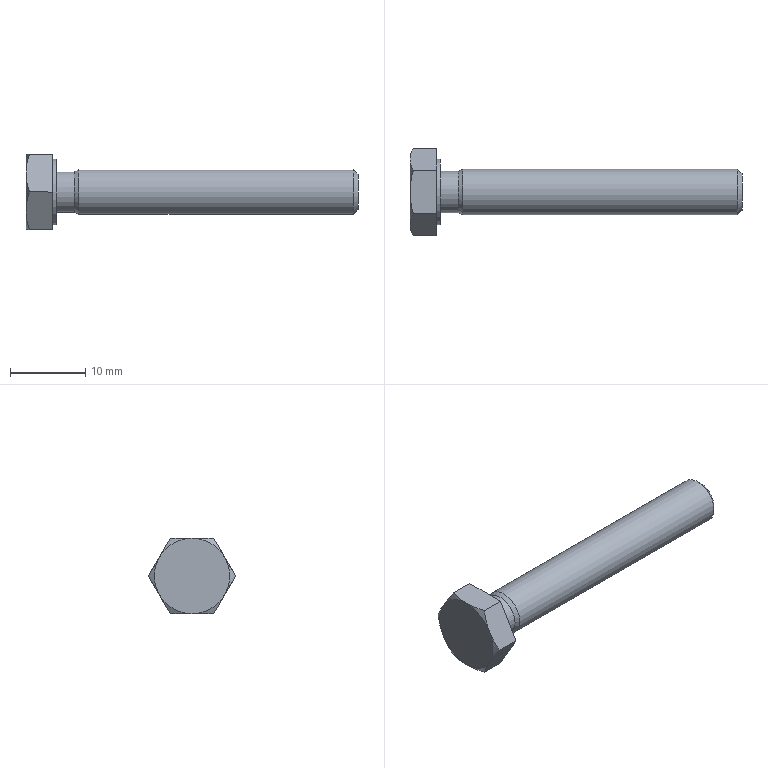Part | STEP file | DIN 933 - M6  x 40 | 1 solid | 21 faces | box 44 x 11.547 x 10 mm | volume 1446 mm3 | plane 10 | cone 8 | cylinder 3 | commonest cylinder face diameters 5.459 x1 6 x1 8.7 x1